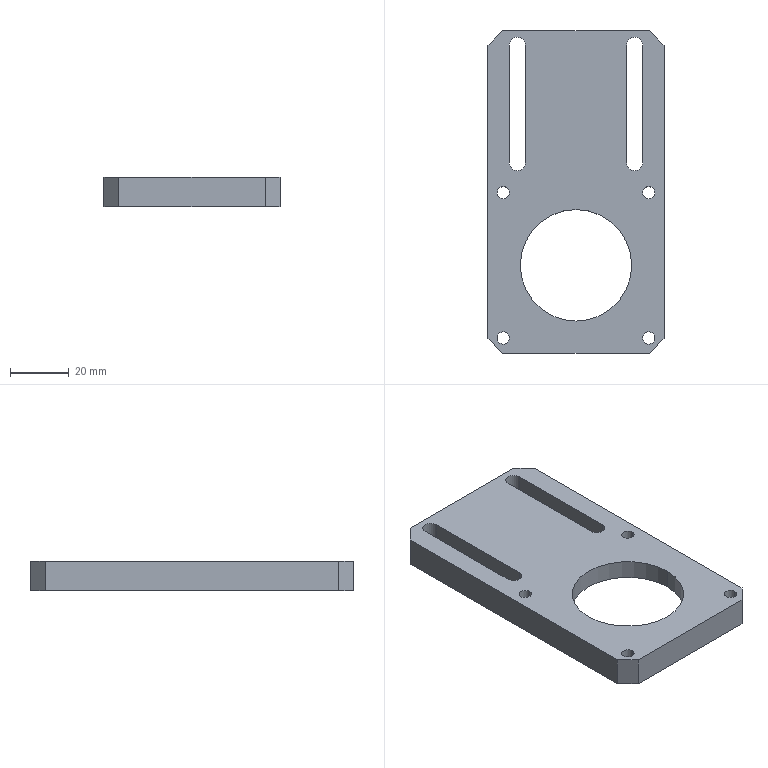Part | SolidWorks | features BaseBody 1 | 1 solid | 31 faces | box 60 x 110 x 10 mm | volume 45827 mm3 | cylinder 16 | plane 15 | commonest cylinder face diameters 4.2 x8 5.5 x4 38 x2 50 x2
STEP:
#1=CARTESIAN_POINT('',(26.849,-0.2513,10.));
#2=VERTEX_POINT('',#1);
#3=CARTESIAN_POINT('',(22.649,-0.2513,10.));
#4=VERTEX_POINT('',#3);
#5=CARTESIAN_POINT('',(24.749,-0.2513,10.));
#6=DIRECTION('',(0.,0.,-1.));
#7=DIRECTION('',(-1.,0.,0.));
#8=AXIS2_PLACEMENT_3D('',#5,#6,#7);
#9=CIRCLE('',#8,2.1);
#10=EDGE_CURVE('',#2,#4,#9,.T.);
#11=ORIENTED_EDGE('',*,*,#10,.F.);
#12=CARTESIAN_POINT('',(26.849,-0.2513,0.));
#13=VERTEX_POINT('',#12);
#14=CARTESIAN_POINT('',(26.849,-0.2513,0.));
#15=DIRECTION('',(0.,0.,-1.));
#16=VECTOR('',#15,1000.);
#17=LINE('',#14,#16);
#18=EDGE_CURVE('',#2,#13,#17,.T.);
#19=ORIENTED_EDGE('',*,*,#18,.T.);
#20=CARTESIAN_POINT('',(22.649,-0.2513,0.));
#21=VERTEX_POINT('',#20);
#22=CARTESIAN_POINT('',(24.749,-0.2513,0.));
#23=DIRECTION('',(0.,0.,-1.));
#24=DIRECTION('',(-1.,0.,0.));
#25=AXIS2_PLACEMENT_3D('',#22,#23,#24);
#26=CIRCLE('',#25,2.1);
#27=EDGE_CURVE('',#13,#21,#26,.T.);
#28=ORIENTED_EDGE('',*,*,#27,.T.);
#29=CARTESIAN_POINT('',(22.649,-0.2513,0.));
#30=DIRECTION('',(0.,0.,-1.));
#31=VECTOR('',#30,1000.);
#32=LINE('',#29,#31);
#33=EDGE_CURVE('',#4,#21,#32,.T.);
#34=ORIENTED_EDGE('',*,*,#33,.F.);
#35=EDGE_LOOP('',(#11,#19,#28,#34));
#36=FACE_OUTER_BOUND('',#35,.T.);
#37=CARTESIAN_POINT('',(24.749,-0.2513,0.));
#38=DIRECTION('',(0.,0.,-1.));
#39=DIRECTION('',(-1.,0.,0.));
#40=AXIS2_PLACEMENT_3D('',#37,#38,#39);
#41=CYLINDRICAL_SURFACE('',#40,2.1);
#42=ADVANCED_FACE('',(#36),#41,.F.);
#43=CARTESIAN_POINT('',(-22.649,-0.2513,10.));
#44=VERTEX_POINT('',#43);
#45=CARTESIAN_POINT('',(-26.849,-0.2513,10.));
#46=VERTEX_POINT('',#45);
#47=CARTESIAN_POINT('',(-24.749,-0.2513,10.));
#48=DIRECTION('',(0.,0.,-1.));
#49=DIRECTION('',(-1.,0.,0.));
#50=AXIS2_PLACEMENT_3D('',#47,#48,#49);
#51=CIRCLE('',#50,2.1);
#52=EDGE_CURVE('',#44,#46,#51,.T.);
#53=ORIENTED_EDGE('',*,*,#52,.F.);
#54=CARTESIAN_POINT('',(-22.649,-0.2513,0.));
#55=VERTEX_POINT('',#54);
#56=CARTESIAN_POINT('',(-22.649,-0.2513,0.));
#57=DIRECTION('',(0.,0.,-1.));
#58=VECTOR('',#57,1000.);
#59=LINE('',#56,#58);
#60=EDGE_CURVE('',#44,#55,#59,.T.);
#61=ORIENTED_EDGE('',*,*,#60,.T.);
#62=CARTESIAN_POINT('',(-26.849,-0.2513,0.));
#63=VERTEX_POINT('',#62);
#64=CARTESIAN_POINT('',(-24.749,-0.2513,0.));
#65=DIRECTION('',(0.,0.,-1.));
#66=DIRECTION('',(-1.,0.,0.));
#67=AXIS2_PLACEMENT_3D('',#64,#65,#66);
#68=CIRCLE('',#67,2.1);
#69=EDGE_CURVE('',#55,#63,#68,.T.);
#70=ORIENTED_EDGE('',*,*,#69,.T.);
#71=CARTESIAN_POINT('',(-26.849,-0.2513,0.));
#72=DIRECTION('',(0.,0.,-1.));
#73=VECTOR('',#72,1000.);
#74=LINE('',#71,#73);
#75=EDGE_CURVE('',#46,#63,#74,.T.);
#76=ORIENTED_EDGE('',*,*,#75,.F.);
#77=EDGE_LOOP('',(#53,#61,#70,#76));
#78=FACE_OUTER_BOUND('',#77,.T.);
#79=CARTESIAN_POINT('',(-24.749,-0.2513,0.));
#80=DIRECTION('',(0.,0.,-1.));
#81=DIRECTION('',(-1.,0.,0.));
#82=AXIS2_PLACEMENT_3D('',#79,#80,#81);
#83=CYLINDRICAL_SURFACE('',#82,2.1);
#84=ADVANCED_FACE('',(#78),#83,.F.);
#85=CARTESIAN_POINT('',(26.849,-49.749,10.));
#86=VERTEX_POINT('',#85);
#87=CARTESIAN_POINT('',(22.649,-49.749,10.));
#88=VERTEX_POINT('',#87);
#89=CARTESIAN_POINT('',(24.749,-49.749,10.));
#90=DIRECTION('',(0.,0.,-1.));
#91=DIRECTION('',(-1.,0.,0.));
#92=AXIS2_PLACEMENT_3D('',#89,#90,#91);
#93=CIRCLE('',#92,2.1);
#94=EDGE_CURVE('',#86,#88,#93,.T.);
#95=ORIENTED_EDGE('',*,*,#94,.F.);
#96=CARTESIAN_POINT('',(26.849,-49.749,0.));
#97=VERTEX_POINT('',#96);
#98=CARTESIAN_POINT('',(26.849,-49.749,0.));
#99=DIRECTION('',(0.,0.,-1.));
#100=VECTOR('',#99,1000.);
#101=LINE('',#98,#100);
#102=EDGE_CURVE('',#86,#97,#101,.T.);
#103=ORIENTED_EDGE('',*,*,#102,.T.);
#104=CARTESIAN_POINT('',(22.649,-49.749,0.));
#105=VERTEX_POINT('',#104);
#106=CARTESIAN_POINT('',(24.749,-49.749,0.));
#107=DIRECTION('',(0.,0.,-1.));
#108=DIRECTION('',(-1.,0.,0.));
#109=AXIS2_PLACEMENT_3D('',#106,#107,#108);
#110=CIRCLE('',#109,2.1);
#111=EDGE_CURVE('',#97,#105,#110,.T.);
#112=ORIENTED_EDGE('',*,*,#111,.T.);
#113=CARTESIAN_POINT('',(22.649,-49.749,0.));
#114=DIRECTION('',(0.,0.,-1.));
#115=VECTOR('',#114,1000.);
#116=LINE('',#113,#115);
#117=EDGE_CURVE('',#88,#105,#116,.T.);
#118=ORIENTED_EDGE('',*,*,#117,.F.);
#119=EDGE_LOOP('',(#95,#103,#112,#118));
#120=FACE_OUTER_BOUND('',#119,.T.);
#121=CARTESIAN_POINT('',(24.749,-49.749,0.));
#122=DIRECTION('',(0.,0.,-1.));
#123=DIRECTION('',(-1.,0.,0.));
#124=AXIS2_PLACEMENT_3D('',#121,#122,#123);
#125=CYLINDRICAL_SURFACE('',#124,2.1);
#126=ADVANCED_FACE('',(#120),#125,.F.);
#127=CARTESIAN_POINT('',(-22.649,-49.749,10.));
#128=VERTEX_POINT('',#127);
#129=CARTESIAN_POINT('',(-26.849,-49.749,10.));
#130=VERTEX_POINT('',#129);
#131=CARTESIAN_POINT('',(-24.749,-49.749,10.));
#132=DIRECTION('',(0.,0.,-1.));
#133=DIRECTION('',(-1.,0.,0.));
#134=AXIS2_PLACEMENT_3D('',#131,#132,#133);
#135=CIRCLE('',#134,2.1);
#136=EDGE_CURVE('',#128,#130,#135,.T.);
#137=ORIENTED_EDGE('',*,*,#136,.F.);
#138=CARTESIAN_POINT('',(-22.649,-49.749,0.));
#139=VERTEX_POINT('',#138);
#140=CARTESIAN_POINT('',(-22.649,-49.749,0.));
#141=DIRECTION('',(0.,0.,-1.));
#142=VECTOR('',#141,1000.);
#143=LINE('',#140,#142);
#144=EDGE_CURVE('',#128,#139,#143,.T.);
#145=ORIENTED_EDGE('',*,*,#144,.T.);
#146=CARTESIAN_POINT('',(-26.849,-49.749,0.));
#147=VERTEX_POINT('',#146);
#148=CARTESIAN_POINT('',(-24.749,-49.749,0.));
#149=DIRECTION('',(0.,0.,-1.));
#150=DIRECTION('',(-1.,0.,0.));
#151=AXIS2_PLACEMENT_3D('',#148,#149,#150);
#152=CIRCLE('',#151,2.1);
#153=EDGE_CURVE('',#139,#147,#152,.T.);
#154=ORIENTED_EDGE('',*,*,#153,.T.);
#155=CARTESIAN_POINT('',(-26.849,-49.749,0.));
#156=DIRECTION('',(0.,0.,-1.));
#157=VECTOR('',#156,1000.);
#158=LINE('',#155,#157);
#159=EDGE_CURVE('',#130,#147,#158,.T.);
#160=ORIENTED_EDGE('',*,*,#159,.F.);
#161=EDGE_LOOP('',(#137,#145,#154,#160));
#162=FACE_OUTER_BOUND('',#161,.T.);
#163=CARTESIAN_POINT('',(-24.749,-49.749,0.));
#164=DIRECTION('',(0.,0.,-1.));
#165=DIRECTION('',(-1.,0.,0.));
#166=AXIS2_PLACEMENT_3D('',#163,#164,#165);
#167=CYLINDRICAL_SURFACE('',#166,2.1);
#168=ADVANCED_FACE('',(#162),#167,.F.);
#169=CARTESIAN_POINT('',(19.,-25.,10.));
#170=VERTEX_POINT('',#169);
#171=CARTESIAN_POINT('',(-19.,-25.,10.));
#172=VERTEX_POINT('',#171);
#173=CARTESIAN_POINT('',(0.,-25.,10.));
#174=DIRECTION('',(0.,0.,-1.));
#175=DIRECTION('',(-1.,0.,0.));
#176=AXIS2_PLACEMENT_3D('',#173,#174,#175);
#177=CIRCLE('',#176,19.);
#178=EDGE_CURVE('',#170,#172,#177,.T.);
#179=ORIENTED_EDGE('',*,*,#178,.F.);
#180=CARTESIAN_POINT('',(19.,-25.,3.5));
#181=VERTEX_POINT('',#180);
#182=CARTESIAN_POINT('',(19.,-25.,10.));
#183=DIRECTION('',(0.,0.,-1.));
#184=VECTOR('',#183,1000.);
#185=LINE('',#182,#184);
#186=EDGE_CURVE('',#170,#181,#185,.T.);
#187=ORIENTED_EDGE('',*,*,#186,.T.);
#188=CARTESIAN_POINT('',(-19.,-25.,3.5));
#189=VERTEX_POINT('',#188);
#190=CARTESIAN_POINT('',(0.,-25.,3.5));
#191=DIRECTION('',(0.,0.,-1.));
#192=DIRECTION('',(-1.,0.,0.));
#193=AXIS2_PLACEMENT_3D('',#190,#191,#192);
#194=CIRCLE('',#193,19.);
#195=EDGE_CURVE('',#181,#189,#194,.T.);
#196=ORIENTED_EDGE('',*,*,#195,.T.);
#197=CARTESIAN_POINT('',(-19.,-25.,10.));
#198=DIRECTION('',(0.,0.,-1.));
#199=VECTOR('',#198,1000.);
#200=LINE('',#197,#199);
#201=EDGE_CURVE('',#172,#189,#200,.T.);
#202=ORIENTED_EDGE('',*,*,#201,.F.);
#203=EDGE_LOOP('',(#179,#187,#196,#202));
#204=FACE_OUTER_BOUND('',#203,.T.);
#205=CARTESIAN_POINT('',(0.,-25.,10.));
#206=DIRECTION('',(0.,0.,-1.));
#207=DIRECTION('',(-1.,0.,0.));
#208=AXIS2_PLACEMENT_3D('',#205,#206,#207);
#209=CYLINDRICAL_SURFACE('',#208,19.);
#210=ADVANCED_FACE('',(#204),#209,.F.);
#211=CARTESIAN_POINT('',(25.,-25.,3.5));
#212=VERTEX_POINT('',#211);
#213=CARTESIAN_POINT('',(-25.,-25.,3.5));
#214=VERTEX_POINT('',#213);
#215=CARTESIAN_POINT('',(0.,-25.,3.5));
#216=DIRECTION('',(0.,0.,-1.));
#217=DIRECTION('',(-1.,0.,0.));
#218=AXIS2_PLACEMENT_3D('',#215,#216,#217);
#219=CIRCLE('',#218,25.);
#220=EDGE_CURVE('',#212,#214,#219,.T.);
#221=ORIENTED_EDGE('',*,*,#220,.F.);
#222=CARTESIAN_POINT('',(25.,-25.,0.));
#223=VERTEX_POINT('',#222);
#224=CARTESIAN_POINT('',(25.,-25.,3.5));
#225=DIRECTION('',(0.,0.,-1.));
#226=VECTOR('',#225,1000.);
#227=LINE('',#224,#226);
#228=EDGE_CURVE('',#212,#223,#227,.T.);
#229=ORIENTED_EDGE('',*,*,#228,.T.);
#230=CARTESIAN_POINT('',(-25.,-25.,0.));
#231=VERTEX_POINT('',#230);
#232=CARTESIAN_POINT('',(0.,-25.,0.));
#233=DIRECTION('',(0.,0.,-1.));
#234=DIRECTION('',(-1.,0.,0.));
#235=AXIS2_PLACEMENT_3D('',#232,#233,#234);
#236=CIRCLE('',#235,25.);
#237=EDGE_CURVE('',#223,#231,#236,.T.);
#238=ORIENTED_EDGE('',*,*,#237,.T.);
#239=CARTESIAN_POINT('',(-25.,-25.,3.5));
#240=DIRECTION('',(0.,0.,-1.));
#241=VECTOR('',#240,1000.);
#242=LINE('',#239,#241);
#243=EDGE_CURVE('',#214,#231,#242,.T.);
#244=ORIENTED_EDGE('',*,*,#243,.F.);
#245=EDGE_LOOP('',(#221,#229,#238,#244));
#246=FACE_OUTER_BOUND('',#245,.T.);
#247=CARTESIAN_POINT('',(0.,-25.,3.5));
#248=DIRECTION('',(0.,0.,-1.));
#249=DIRECTION('',(-1.,0.,0.));
#250=AXIS2_PLACEMENT_3D('',#247,#248,#249);
#251=CYLINDRICAL_SURFACE('',#250,25.);
#252=ADVANCED_FACE('',(#246),#251,.F.);
#253=CARTESIAN_POINT('',(-30.,50.,10.));
#254=VERTEX_POINT('',#253);
#255=CARTESIAN_POINT('',(-30.,-50.,10.));
#256=VERTEX_POINT('',#255);
#257=CARTESIAN_POINT('',(-30.,55.,10.));
#258=DIRECTION('',(0.,-1.,0.));
#259=VECTOR('',#258,1000.);
#260=LINE('',#257,#259);
#261=EDGE_CURVE('',#254,#256,#260,.T.);
#262=ORIENTED_EDGE('',*,*,#261,.F.);
#263=CARTESIAN_POINT('',(-30.,50.,0.));
#264=VERTEX_POINT('',#263);
#265=CARTESIAN_POINT('',(-30.,50.,10.));
#266=DIRECTION('',(0.,0.,-1.));
#267=VECTOR('',#266,1000.);
#268=LINE('',#265,#267);
#269=EDGE_CURVE('',#254,#264,#268,.T.);
#270=ORIENTED_EDGE('',*,*,#269,.T.);
#271=CARTESIAN_POINT('',(-30.,-50.,0.));
#272=VERTEX_POINT('',#271);
#273=CARTESIAN_POINT('',(-30.,55.,0.));
#274=DIRECTION('',(0.,-1.,0.));
#275=VECTOR('',#274,1000.);
#276=LINE('',#273,#275);
#277=EDGE_CURVE('',#264,#272,#276,.T.);
#278=ORIENTED_EDGE('',*,*,#277,.T.);
#279=CARTESIAN_POINT('',(-30.,-50.,10.));
#280=DIRECTION('',(0.,0.,1.));
#281=VECTOR('',#280,1000.);
#282=LINE('',#279,#281);
#283=EDGE_CURVE('',#272,#256,#282,.T.);
#284=ORIENTED_EDGE('',*,*,#283,.T.);
#285=EDGE_LOOP('',(#262,#270,#278,#284));
#286=FACE_OUTER_BOUND('',#285,.T.);
#287=CARTESIAN_POINT('',(-30.,55.,10.));
#288=DIRECTION('',(1.,0.,0.));
#289=DIRECTION('',(0.,1.,0.));
#290=AXIS2_PLACEMENT_3D('',#287,#288,#289);
#291=PLANE('',#290);
#292=ADVANCED_FACE('',(#286),#291,.F.);
#293=CARTESIAN_POINT('',(-25.,-55.,0.));
#294=VERTEX_POINT('',#293);
#295=CARTESIAN_POINT('',(25.,-55.,0.));
#296=VERTEX_POINT('',#295);
#297=CARTESIAN_POINT('',(30.,-55.,0.));
#298=DIRECTION('',(1.,0.,0.));
#299=VECTOR('',#298,1000.);
#300=LINE('',#297,#299);
#301=EDGE_CURVE('',#294,#296,#300,.T.);
#302=ORIENTED_EDGE('',*,*,#301,.T.);
#303=CARTESIAN_POINT('',(25.,-55.,10.));
#304=VERTEX_POINT('',#303);
#305=CARTESIAN_POINT('',(25.,-55.,10.));
#306=DIRECTION('',(0.,0.,1.));
#307=VECTOR('',#306,1000.);
#308=LINE('',#305,#307);
#309=EDGE_CURVE('',#296,#304,#308,.T.);
#310=ORIENTED_EDGE('',*,*,#309,.T.);
#311=CARTESIAN_POINT('',(-25.,-55.,10.));
#312=VERTEX_POINT('',#311);
#313=CARTESIAN_POINT('',(30.,-55.,10.));
#314=DIRECTION('',(1.,0.,0.));
#315=VECTOR('',#314,1000.);
#316=LINE('',#313,#315);
#317=EDGE_CURVE('',#312,#304,#316,.T.);
#318=ORIENTED_EDGE('',*,*,#317,.F.);
#319=CARTESIAN_POINT('',(-25.,-55.,10.));
#320=DIRECTION('',(0.,0.,-1.));
#321=VECTOR('',#320,1000.);
#322=LINE('',#319,#321);
#323=EDGE_CURVE('',#312,#294,#322,.T.);
#324=ORIENTED_EDGE('',*,*,#323,.T.);
#325=EDGE_LOOP('',(#302,#310,#318,#324));
#326=FACE_OUTER_BOUND('',#325,.T.);
#327=CARTESIAN_POINT('',(30.,-55.,10.));
#328=DIRECTION('',(0.,1.,0.));
#329=DIRECTION('',(-1.,0.,0.));
#330=AXIS2_PLACEMENT_3D('',#327,#328,#329);
#331=PLANE('',#330);
#332=ADVANCED_FACE('',(#326),#331,.F.);
#333=CARTESIAN_POINT('',(30.,-50.,0.));
#334=VERTEX_POINT('',#333);
#335=CARTESIAN_POINT('',(30.,50.,0.));
#336=VERTEX_POINT('',#335);
#337=CARTESIAN_POINT('',(30.,55.,0.));
#338=DIRECTION('',(0.,1.,0.));
#339=VECTOR('',#338,1000.);
#340=LINE('',#337,#339);
#341=EDGE_CURVE('',#334,#336,#340,.T.);
#342=ORIENTED_EDGE('',*,*,#341,.T.);
#343=CARTESIAN_POINT('',(30.,50.,10.));
#344=VERTEX_POINT('',#343);
#345=CARTESIAN_POINT('',(30.,50.,10.));
#346=DIRECTION('',(0.,0.,1.));
#347=VECTOR('',#346,1000.);
#348=LINE('',#345,#347);
#349=EDGE_CURVE('',#336,#344,#348,.T.);
#350=ORIENTED_EDGE('',*,*,#349,.T.);
#351=CARTESIAN_POINT('',(30.,-50.,10.));
#352=VERTEX_POINT('',#351);
#353=CARTESIAN_POINT('',(30.,55.,10.));
#354=DIRECTION('',(0.,1.,0.));
#355=VECTOR('',#354,1000.);
#356=LINE('',#353,#355);
#357=EDGE_CURVE('',#352,#344,#356,.T.);
#358=ORIENTED_EDGE('',*,*,#357,.F.);
#359=CARTESIAN_POINT('',(30.,-50.,10.));
#360=DIRECTION('',(0.,0.,-1.));
#361=VECTOR('',#360,1000.);
#362=LINE('',#359,#361);
#363=EDGE_CURVE('',#352,#334,#362,.T.);
#364=ORIENTED_EDGE('',*,*,#363,.T.);
#365=EDGE_LOOP('',(#342,#350,#358,#364));
#366=FACE_OUTER_BOUND('',#365,.T.);
#367=CARTESIAN_POINT('',(30.,55.,10.));
#368=DIRECTION('',(-1.,0.,0.));
#369=DIRECTION('',(0.,-1.,0.));
#370=AXIS2_PLACEMENT_3D('',#367,#368,#369);
#371=PLANE('',#370);
#372=ADVANCED_FACE('',(#366),#371,.F.);
#373=CARTESIAN_POINT('',(25.,55.,10.));
#374=VERTEX_POINT('',#373);
#375=CARTESIAN_POINT('',(-25.,55.,10.));
#376=VERTEX_POINT('',#375);
#377=CARTESIAN_POINT('',(30.,55.,10.));
#378=DIRECTION('',(-1.,0.,0.));
#379=VECTOR('',#378,1000.);
#380=LINE('',#377,#379);
#381=EDGE_CURVE('',#374,#376,#380,.T.);
#382=ORIENTED_EDGE('',*,*,#381,.F.);
#383=CARTESIAN_POINT('',(25.,55.,0.));
#384=VERTEX_POINT('',#383);
#385=CARTESIAN_POINT('',(25.,55.,10.));
#386=DIRECTION('',(0.,0.,-1.));
#387=VECTOR('',#386,1000.);
#388=LINE('',#385,#387);
#389=EDGE_CURVE('',#374,#384,#388,.T.);
#390=ORIENTED_EDGE('',*,*,#389,.T.);
#391=CARTESIAN_POINT('',(-25.,55.,0.));
#392=VERTEX_POINT('',#391);
#393=CARTESIAN_POINT('',(30.,55.,0.));
#394=DIRECTION('',(-1.,0.,0.));
#395=VECTOR('',#394,1000.);
#396=LINE('',#393,#395);
#397=EDGE_CURVE('',#384,#392,#396,.T.);
#398=ORIENTED_EDGE('',*,*,#397,.T.);
#399=CARTESIAN_POINT('',(-25.,55.,10.));
#400=DIRECTION('',(0.,0.,1.));
#401=VECTOR('',#400,1000.);
#402=LINE('',#399,#401);
#403=EDGE_CURVE('',#392,#376,#402,.T.);
#404=ORIENTED_EDGE('',*,*,#403,.T.);
#405=EDGE_LOOP('',(#382,#390,#398,#404));
#406=FACE_OUTER_BOUND('',#405,.T.);
#407=CARTESIAN_POINT('',(30.,55.,10.));
#408=DIRECTION('',(0.,-1.,0.));
#409=DIRECTION('',(1.,0.,0.));
#410=AXIS2_PLACEMENT_3D('',#407,#408,#409);
#411=PLANE('',#410);
#412=ADVANCED_FACE('',(#406),#411,.F.);
#413=CARTESIAN_POINT('',(24.749,-0.2513,10.));
#414=DIRECTION('',(0.,0.,-1.));
#415=DIRECTION('',(-1.,0.,0.));
#416=AXIS2_PLACEMENT_3D('',#413,#414,#415);
#417=CIRCLE('',#416,2.1);
#418=EDGE_CURVE('',#4,#2,#417,.T.);
#419=ORIENTED_EDGE('',*,*,#418,.T.);
#420=ORIENTED_EDGE('',*,*,#10,.T.);
#421=EDGE_LOOP('',(#419,#420));
#422=FACE_BOUND('',#421,.T.);
#423=CARTESIAN_POINT('',(-24.749,-0.2513,10.));
#424=DIRECTION('',(0.,0.,-1.));
#425=DIRECTION('',(-1.,0.,0.));
#426=AXIS2_PLACEMENT_3D('',#423,#424,#425);
#427=CIRCLE('',#426,2.1);
#428=EDGE_CURVE('',#46,#44,#427,.T.);
#429=ORIENTED_EDGE('',*,*,#428,.T.);
#430=ORIENTED_EDGE('',*,*,#52,.T.);
#431=EDGE_LOOP('',(#429,#430));
#432=FACE_BOUND('',#431,.T.);
#433=CARTESIAN_POINT('',(24.749,-49.749,10.));
#434=DIRECTION('',(0.,0.,-1.));
#435=DIRECTION('',(-1.,0.,0.));
#436=AXIS2_PLACEMENT_3D('',#433,#434,#435);
#437=CIRCLE('',#436,2.1);
#438=EDGE_CURVE('',#88,#86,#437,.T.);
#439=ORIENTED_EDGE('',*,*,#438,.T.);
#440=ORIENTED_EDGE('',*,*,#94,.T.);
#441=EDGE_LOOP('',(#439,#440));
#442=FACE_BOUND('',#441,.T.);
#443=CARTESIAN_POINT('',(-24.749,-49.749,10.));
#444=DIRECTION('',(0.,0.,-1.));
#445=DIRECTION('',(-1.,0.,0.));
#446=AXIS2_PLACEMENT_3D('',#443,#444,#445);
#447=CIRCLE('',#446,2.1);
#448=EDGE_CURVE('',#130,#128,#447,.T.);
#449=ORIENTED_EDGE('',*,*,#448,.T.);
#450=ORIENTED_EDGE('',*,*,#136,.T.);
#451=EDGE_LOOP('',(#449,#450));
#452=FACE_BOUND('',#451,.T.);
#453=CARTESIAN_POINT('',(17.25,50.,10.));
#454=VERTEX_POINT('',#453);
#455=CARTESIAN_POINT('',(17.25,10.,10.));
#456=VERTEX_POINT('',#455);
#457=CARTESIAN_POINT('',(17.25,50.,10.));
#458=DIRECTION('',(0.,-1.,0.));
#459=VECTOR('',#458,1000.);
#460=LINE('',#457,#459);
#461=EDGE_CURVE('',#454,#456,#460,.T.);
#462=ORIENTED_EDGE('',*,*,#461,.F.);
#463=CARTESIAN_POINT('',(22.75,50.,10.));
#464=VERTEX_POINT('',#463);
#465=CARTESIAN_POINT('',(20.,50.,10.));
#466=DIRECTION('',(0.,0.,1.));
#467=DIRECTION('',(-1.,0.,0.));
#468=AXIS2_PLACEMENT_3D('',#465,#466,#467);
#469=CIRCLE('',#468,2.75);
#470=EDGE_CURVE('',#464,#454,#469,.T.);
#471=ORIENTED_EDGE('',*,*,#470,.F.);
#472=CARTESIAN_POINT('',(22.75,10.,10.));
#473=VERTEX_POINT('',#472);
#474=CARTESIAN_POINT('',(22.75,50.,10.));
#475=DIRECTION('',(0.,1.,0.));
#476=VECTOR('',#475,1000.);
#477=LINE('',#474,#476);
#478=EDGE_CURVE('',#473,#464,#477,.T.);
#479=ORIENTED_EDGE('',*,*,#478,.F.);
#480=CARTESIAN_POINT('',(20.,10.,10.));
#481=DIRECTION('',(0.,0.,1.));
#482=DIRECTION('',(-1.,0.,0.));
#483=AXIS2_PLACEMENT_3D('',#480,#481,#482);
#484=CIRCLE('',#483,2.75);
#485=EDGE_CURVE('',#456,#473,#484,.T.);
#486=ORIENTED_EDGE('',*,*,#485,.F.);
#487=EDGE_LOOP('',(#462,#471,#479,#486));
#488=FACE_BOUND('',#487,.T.);
#489=CARTESIAN_POINT('',(-22.75,50.,10.));
#490=VERTEX_POINT('',#489);
#491=CARTESIAN_POINT('',(-22.75,10.,10.));
#492=VERTEX_POINT('',#491);
#493=CARTESIAN_POINT('',(-22.75,50.,10.));
#494=DIRECTION('',(0.,-1.,0.));
#495=VECTOR('',#494,1000.);
#496=LINE('',#493,#495);
#497=EDGE_CURVE('',#490,#492,#496,.T.);
#498=ORIENTED_EDGE('',*,*,#497,.F.);
#499=CARTESIAN_POINT('',(-17.25,50.,10.));
#500=VERTEX_POINT('',#499);
#501=CARTESIAN_POINT('',(-20.,50.,10.));
#502=DIRECTION('',(0.,0.,1.));
#503=DIRECTION('',(1.,0.,0.));
#504=AXIS2_PLACEMENT_3D('',#501,#502,#503);
#505=CIRCLE('',#504,2.75);
#506=EDGE_CURVE('',#500,#490,#505,.T.);
#507=ORIENTED_EDGE('',*,*,#506,.F.);
#508=CARTESIAN_POINT('',(-17.25,10.,10.));
#509=VERTEX_POINT('',#508);
#510=CARTESIAN_POINT('',(-17.25,50.,10.));
#511=DIRECTION('',(0.,1.,0.));
#512=VECTOR('',#511,1000.);
#513=LINE('',#510,#512);
#514=EDGE_CURVE('',#509,#500,#513,.T.);
#515=ORIENTED_EDGE('',*,*,#514,.F.);
#516=CARTESIAN_POINT('',(-20.,10.,10.));
#517=DIRECTION('',(0.,0.,1.));
#518=DIRECTION('',(1.,0.,0.));
#519=AXIS2_PLACEMENT_3D('',#516,#517,#518);
#520=CIRCLE('',#519,2.75);
#521=EDGE_CURVE('',#492,#509,#520,.T.);
#522=ORIENTED_EDGE('',*,*,#521,.F.);
#523=EDGE_LOOP('',(#498,#507,#515,#522));
#524=FACE_BOUND('',#523,.T.);
#525=CARTESIAN_POINT('',(0.,-25.,10.));
#526=DIRECTION('',(0.,0.,-1.));
#527=DIRECTION('',(-1.,0.,0.));
#528=AXIS2_PLACEMENT_3D('',#525,#526,#527);
#529=CIRCLE('',#528,19.);
#530=EDGE_CURVE('',#172,#170,#529,.T.);
#531=ORIENTED_EDGE('',*,*,#530,.T.);
#532=ORIENTED_EDGE('',*,*,#178,.T.);
#533=EDGE_LOOP('',(#531,#532));
#534=FACE_BOUND('',#533,.T.);
#535=ORIENTED_EDGE('',*,*,#357,.T.);
#536=CARTESIAN_POINT('',(25.,55.,10.));
#537=DIRECTION('',(-0.7071,0.7071,0.));
#538=VECTOR('',#537,1000.);
#539=LINE('',#536,#538);
#540=EDGE_CURVE('',#344,#374,#539,.T.);
#541=ORIENTED_EDGE('',*,*,#540,.T.);
#542=ORIENTED_EDGE('',*,*,#381,.T.);
#543=CARTESIAN_POINT('',(-30.,50.,10.));
#544=DIRECTION('',(-0.7071,-0.7071,0.));
#545=VECTOR('',#544,1000.);
#546=LINE('',#543,#545);
#547=EDGE_CURVE('',#376,#254,#546,.T.);
#548=ORIENTED_EDGE('',*,*,#547,.T.);
#549=ORIENTED_EDGE('',*,*,#261,.T.);
#550=CARTESIAN_POINT('',(-25.,-55.,10.));
#551=DIRECTION('',(0.7071,-0.7071,0.));
#552=VECTOR('',#551,1000.);
#553=LINE('',#550,#552);
#554=EDGE_CURVE('',#256,#312,#553,.T.);
#555=ORIENTED_EDGE('',*,*,#554,.T.);
#556=ORIENTED_EDGE('',*,*,#317,.T.);
#557=CARTESIAN_POINT('',(30.,-50.,10.));
#558=DIRECTION('',(0.7071,0.7071,0.));
#559=VECTOR('',#558,1000.);
#560=LINE('',#557,#559);
#561=EDGE_CURVE('',#304,#352,#560,.T.);
#562=ORIENTED_EDGE('',*,*,#561,.T.);
#563=EDGE_LOOP('',(#535,#541,#542,#548,#549,#555,#556,#562));
#564=FACE_OUTER_BOUND('',#563,.T.);
#565=CARTESIAN_POINT('',(0.,0.,10.));
#566=DIRECTION('',(0.,0.,-1.));
#567=DIRECTION('',(-1.,0.,0.));
#568=AXIS2_PLACEMENT_3D('',#565,#566,#567);
#569=PLANE('',#568);
#570=ADVANCED_FACE('',(#422,#432,#442,#452,#488,#524,#534,#564),#569,.F.);
#571=CARTESIAN_POINT('',(24.749,-0.2513,0.));
#572=DIRECTION('',(0.,0.,-1.));
#573=DIRECTION('',(-1.,0.,0.));
#574=AXIS2_PLACEMENT_3D('',#571,#572,#573);
#575=CIRCLE('',#574,2.1);
#576=EDGE_CURVE('',#21,#13,#575,.T.);
#577=ORIENTED_EDGE('',*,*,#576,.F.);
#578=ORIENTED_EDGE('',*,*,#27,.F.);
#579=EDGE_LOOP('',(#577,#578));
#580=FACE_BOUND('',#579,.T.);
#581=CARTESIAN_POINT('',(-24.749,-0.2513,0.));
#582=DIRECTION('',(0.,0.,-1.));
#583=DIRECTION('',(-1.,0.,0.));
#584=AXIS2_PLACEMENT_3D('',#581,#582,#583);
#585=CIRCLE('',#584,2.1);
#586=EDGE_CURVE('',#63,#55,#585,.T.);
#587=ORIENTED_EDGE('',*,*,#586,.F.);
#588=ORIENTED_EDGE('',*,*,#69,.F.);
#589=EDGE_LOOP('',(#587,#588));
#590=FACE_BOUND('',#589,.T.);
#591=CARTESIAN_POINT('',(24.749,-49.749,0.));
#592=DIRECTION('',(0.,0.,-1.));
#593=DIRECTION('',(-1.,0.,0.));
#594=AXIS2_PLACEMENT_3D('',#591,#592,#593);
#595=CIRCLE('',#594,2.1);
#596=EDGE_CURVE('',#105,#97,#595,.T.);
#597=ORIENTED_EDGE('',*,*,#596,.F.);
#598=ORIENTED_EDGE('',*,*,#111,.F.);
#599=EDGE_LOOP('',(#597,#598));
#600=FACE_BOUND('',#599,.T.);
#601=CARTESIAN_POINT('',(-24.749,-49.749,0.));
#602=DIRECTION('',(0.,0.,-1.));
#603=DIRECTION('',(-1.,0.,0.));
#604=AXIS2_PLACEMENT_3D('',#601,#602,#603);
#605=CIRCLE('',#604,2.1);
#606=EDGE_CURVE('',#147,#139,#605,.T.);
#607=ORIENTED_EDGE('',*,*,#606,.F.);
#608=ORIENTED_EDGE('',*,*,#153,.F.);
#609=EDGE_LOOP('',(#607,#608));
#610=FACE_BOUND('',#609,.T.);
#611=CARTESIAN_POINT('',(22.75,50.,0.));
#612=VERTEX_POINT('',#611);
#613=CARTESIAN_POINT('',(17.25,50.,0.));
#614=VERTEX_POINT('',#613);
#615=CARTESIAN_POINT('',(20.,50.,0.));
#616=DIRECTION('',(0.,0.,1.));
#617=DIRECTION('',(-1.,0.,0.));
#618=AXIS2_PLACEMENT_3D('',#615,#616,#617);
#619=CIRCLE('',#618,2.75);
#620=EDGE_CURVE('',#612,#614,#619,.T.);
#621=ORIENTED_EDGE('',*,*,#620,.T.);
#622=CARTESIAN_POINT('',(17.25,10.,0.));
#623=VERTEX_POINT('',#622);
#624=CARTESIAN_POINT('',(17.25,50.,0.));
#625=DIRECTION('',(0.,-1.,0.));
#626=VECTOR('',#625,1000.);
#627=LINE('',#624,#626);
#628=EDGE_CURVE('',#614,#623,#627,.T.);
#629=ORIENTED_EDGE('',*,*,#628,.T.);
#630=CARTESIAN_POINT('',(22.75,10.,0.));
#631=VERTEX_POINT('',#630);
#632=CARTESIAN_POINT('',(20.,10.,0.));
#633=DIRECTION('',(0.,0.,1.));
#634=DIRECTION('',(-1.,0.,0.));
#635=AXIS2_PLACEMENT_3D('',#632,#633,#634);
#636=CIRCLE('',#635,2.75);
#637=EDGE_CURVE('',#623,#631,#636,.T.);
#638=ORIENTED_EDGE('',*,*,#637,.T.);
#639=CARTESIAN_POINT('',(22.75,50.,0.));
#640=DIRECTION('',(0.,1.,0.));
#641=VECTOR('',#640,1000.);
#642=LINE('',#639,#641);
#643=EDGE_CURVE('',#631,#612,#642,.T.);
#644=ORIENTED_EDGE('',*,*,#643,.T.);
#645=EDGE_LOOP('',(#621,#629,#638,#644));
#646=FACE_BOUND('',#645,.T.);
#647=CARTESIAN_POINT('',(-17.25,50.,0.));
#648=VERTEX_POINT('',#647);
#649=CARTESIAN_POINT('',(-22.75,50.,0.));
#650=VERTEX_POINT('',#649);
#651=CARTESIAN_POINT('',(-20.,50.,0.));
#652=DIRECTION('',(0.,0.,1.));
#653=DIRECTION('',(1.,0.,0.));
#654=AXIS2_PLACEMENT_3D('',#651,#652,#653);
#655=CIRCLE('',#654,2.75);
#656=EDGE_CURVE('',#648,#650,#655,.T.);
#657=ORIENTED_EDGE('',*,*,#656,.T.);
#658=CARTESIAN_POINT('',(-22.75,10.,0.));
#659=VERTEX_POINT('',#658);
#660=CARTESIAN_POINT('',(-22.75,50.,0.));
#661=DIRECTION('',(0.,-1.,0.));
#662=VECTOR('',#661,1000.);
#663=LINE('',#660,#662);
#664=EDGE_CURVE('',#650,#659,#663,.T.);
#665=ORIENTED_EDGE('',*,*,#664,.T.);
#666=CARTESIAN_POINT('',(-17.25,10.,0.));
#667=VERTEX_POINT('',#666);
#668=CARTESIAN_POINT('',(-20.,10.,0.));
#669=DIRECTION('',(0.,0.,1.));
#670=DIRECTION('',(1.,0.,0.));
#671=AXIS2_PLACEMENT_3D('',#668,#669,#670);
#672=CIRCLE('',#671,2.75);
#673=EDGE_CURVE('',#659,#667,#672,.T.);
#674=ORIENTED_EDGE('',*,*,#673,.T.);
#675=CARTESIAN_POINT('',(-17.25,50.,0.));
#676=DIRECTION('',(0.,1.,0.));
#677=VECTOR('',#676,1000.);
#678=LINE('',#675,#677);
#679=EDGE_CURVE('',#667,#648,#678,.T.);
#680=ORIENTED_EDGE('',*,*,#679,.T.);
#681=EDGE_LOOP('',(#657,#665,#674,#680));
#682=FACE_BOUND('',#681,.T.);
#683=CARTESIAN_POINT('',(0.,-25.,0.));
#684=DIRECTION('',(0.,0.,-1.));
#685=DIRECTION('',(-1.,0.,0.));
#686=AXIS2_PLACEMENT_3D('',#683,#684,#685);
#687=CIRCLE('',#686,25.);
#688=EDGE_CURVE('',#231,#223,#687,.T.);
#689=ORIENTED_EDGE('',*,*,#688,.F.);
#690=ORIENTED_EDGE('',*,*,#237,.F.);
#691=EDGE_LOOP('',(#689,#690));
#692=FACE_BOUND('',#691,.T.);
#693=ORIENTED_EDGE('',*,*,#397,.F.);
#694=CARTESIAN_POINT('',(40.,40.,0.));
#695=DIRECTION('',(0.7071,-0.7071,0.));
#696=VECTOR('',#695,1000.);
#697=LINE('',#694,#696);
#698=EDGE_CURVE('',#384,#336,#697,.T.);
#699=ORIENTED_EDGE('',*,*,#698,.T.);
#700=ORIENTED_EDGE('',*,*,#341,.F.);
#701=CARTESIAN_POINT('',(40.,-40.,0.));
#702=DIRECTION('',(-0.7071,-0.7071,0.));
#703=VECTOR('',#702,1000.);
#704=LINE('',#701,#703);
#705=EDGE_CURVE('',#334,#296,#704,.T.);
#706=ORIENTED_EDGE('',*,*,#705,.T.);
#707=ORIENTED_EDGE('',*,*,#301,.F.);
#708=CARTESIAN_POINT('',(-40.,-40.,0.));
#709=DIRECTION('',(-0.7071,0.7071,0.));
#710=VECTOR('',#709,1000.);
#711=LINE('',#708,#710);
#712=EDGE_CURVE('',#294,#272,#711,.T.);
#713=ORIENTED_EDGE('',*,*,#712,.T.);
#714=ORIENTED_EDGE('',*,*,#277,.F.);
#715=CARTESIAN_POINT('',(-40.,40.,0.));
#716=DIRECTION('',(0.7071,0.7071,0.));
#717=VECTOR('',#716,1000.);
#718=LINE('',#715,#717);
#719=EDGE_CURVE('',#264,#392,#718,.T.);
#720=ORIENTED_EDGE('',*,*,#719,.T.);
#721=EDGE_LOOP('',(#693,#699,#700,#706,#707,#713,#714,#720));
#722=FACE_OUTER_BOUND('',#721,.T.);
#723=CARTESIAN_POINT('',(0.,0.,0.));
#724=DIRECTION('',(0.,0.,-1.));
#725=DIRECTION('',(-1.,0.,0.));
#726=AXIS2_PLACEMENT_3D('',#723,#724,#725);
#727=PLANE('',#726);
#728=ADVANCED_FACE('',(#580,#590,#600,#610,#646,#682,#692,#722),#727,.T.);
#729=ORIENTED_EDGE('',*,*,#228,.F.);
#730=CARTESIAN_POINT('',(0.,-25.,3.5));
#731=DIRECTION('',(0.,0.,-1.));
#732=DIRECTION('',(-1.,0.,0.));
#733=AXIS2_PLACEMENT_3D('',#730,#731,#732);
#734=CIRCLE('',#733,25.);
#735=EDGE_CURVE('',#214,#212,#734,.T.);
#736=ORIENTED_EDGE('',*,*,#735,.F.);
#737=ORIENTED_EDGE('',*,*,#243,.T.);
#738=ORIENTED_EDGE('',*,*,#688,.T.);
#739=EDGE_LOOP('',(#729,#736,#737,#738));
#740=FACE_OUTER_BOUND('',#739,.T.);
#741=CARTESIAN_POINT('',(0.,-25.,3.5));
#742=DIRECTION('',(0.,0.,-1.));
#743=DIRECTION('',(-1.,0.,0.));
#744=AXIS2_PLACEMENT_3D('',#741,#742,#743);
#745=CYLINDRICAL_SURFACE('',#744,25.);
#746=ADVANCED_FACE('',(#740),#745,.F.);
#747=CARTESIAN_POINT('',(0.,-25.,3.5));
#748=DIRECTION('',(0.,0.,-1.));
#749=DIRECTION('',(-1.,0.,0.));
#750=AXIS2_PLACEMENT_3D('',#747,#748,#749);
#751=CIRCLE('',#750,19.);
#752=EDGE_CURVE('',#189,#181,#751,.T.);
#753=ORIENTED_EDGE('',*,*,#752,.F.);
#754=ORIENTED_EDGE('',*,*,#195,.F.);
#755=EDGE_LOOP('',(#753,#754));
#756=FACE_BOUND('',#755,.T.);
#757=ORIENTED_EDGE('',*,*,#735,.T.);
#758=ORIENTED_EDGE('',*,*,#220,.T.);
#759=EDGE_LOOP('',(#757,#758));
#760=FACE_OUTER_BOUND('',#759,.T.);
#761=CARTESIAN_POINT('',(0.,-25.,3.5));
#762=DIRECTION('',(0.,0.,-1.));
#763=DIRECTION('',(-1.,0.,0.));
#764=AXIS2_PLACEMENT_3D('',#761,#762,#763);
#765=PLANE('',#764);
#766=ADVANCED_FACE('',(#756,#760),#765,.T.);
#767=ORIENTED_EDGE('',*,*,#186,.F.);
#768=ORIENTED_EDGE('',*,*,#530,.F.);
#769=ORIENTED_EDGE('',*,*,#201,.T.);
#770=ORIENTED_EDGE('',*,*,#752,.T.);
#771=EDGE_LOOP('',(#767,#768,#769,#770));
#772=FACE_OUTER_BOUND('',#771,.T.);
#773=CARTESIAN_POINT('',(0.,-25.,10.));
#774=DIRECTION('',(0.,0.,-1.));
#775=DIRECTION('',(-1.,0.,0.));
#776=AXIS2_PLACEMENT_3D('',#773,#774,#775);
#777=CYLINDRICAL_SURFACE('',#776,19.);
#778=ADVANCED_FACE('',(#772),#777,.F.);
#779=ORIENTED_EDGE('',*,*,#540,.F.);
#780=ORIENTED_EDGE('',*,*,#349,.F.);
#781=ORIENTED_EDGE('',*,*,#698,.F.);
#782=ORIENTED_EDGE('',*,*,#389,.F.);
#783=EDGE_LOOP('',(#779,#780,#781,#782));
#784=FACE_OUTER_BOUND('',#783,.T.);
#785=CARTESIAN_POINT('',(25.,55.,10.));
#786=DIRECTION('',(-0.7071,-0.7071,0.));
#787=DIRECTION('',(0.,0.,-1.));
#788=AXIS2_PLACEMENT_3D('',#785,#786,#787);
#789=PLANE('',#788);
#790=ADVANCED_FACE('',(#784),#789,.F.);
#791=ORIENTED_EDGE('',*,*,#547,.F.);
#792=ORIENTED_EDGE('',*,*,#403,.F.);
#793=ORIENTED_EDGE('',*,*,#719,.F.);
#794=ORIENTED_EDGE('',*,*,#269,.F.);
#795=EDGE_LOOP('',(#791,#792,#793,#794));
#796=FACE_OUTER_BOUND('',#795,.T.);
#797=CARTESIAN_POINT('',(-30.,50.,10.));
#798=DIRECTION('',(0.7071,-0.7071,0.));
#799=DIRECTION('',(0.,0.,-1.));
#800=AXIS2_PLACEMENT_3D('',#797,#798,#799);
#801=PLANE('',#800);
#802=ADVANCED_FACE('',(#796),#801,.F.);
#803=ORIENTED_EDGE('',*,*,#561,.F.);
#804=ORIENTED_EDGE('',*,*,#309,.F.);
#805=ORIENTED_EDGE('',*,*,#705,.F.);
#806=ORIENTED_EDGE('',*,*,#363,.F.);
#807=EDGE_LOOP('',(#803,#804,#805,#806));
#808=FACE_OUTER_BOUND('',#807,.T.);
#809=CARTESIAN_POINT('',(30.,-50.,10.));
#810=DIRECTION('',(-0.7071,0.7071,0.));
#811=DIRECTION('',(0.,0.,-1.));
#812=AXIS2_PLACEMENT_3D('',#809,#810,#811);
#813=PLANE('',#812);
#814=ADVANCED_FACE('',(#808),#813,.F.);
#815=ORIENTED_EDGE('',*,*,#554,.F.);
#816=ORIENTED_EDGE('',*,*,#283,.F.);
#817=ORIENTED_EDGE('',*,*,#712,.F.);
#818=ORIENTED_EDGE('',*,*,#323,.F.);
#819=EDGE_LOOP('',(#815,#816,#817,#818));
#820=FACE_OUTER_BOUND('',#819,.T.);
#821=CARTESIAN_POINT('',(-25.,-55.,10.));
#822=DIRECTION('',(0.7071,0.7071,0.));
#823=DIRECTION('',(0.,0.,-1.));
#824=AXIS2_PLACEMENT_3D('',#821,#822,#823);
#825=PLANE('',#824);
#826=ADVANCED_FACE('',(#820),#825,.F.);
#827=ORIENTED_EDGE('',*,*,#506,.T.);
#828=CARTESIAN_POINT('',(-22.75,50.,0.));
#829=DIRECTION('',(0.,0.,1.));
#830=VECTOR('',#829,1000.);
#831=LINE('',#828,#830);
#832=EDGE_CURVE('',#650,#490,#831,.T.);
#833=ORIENTED_EDGE('',*,*,#832,.F.);
#834=ORIENTED_EDGE('',*,*,#656,.F.);
#835=CARTESIAN_POINT('',(-17.25,50.,0.));
#836=DIRECTION('',(0.,0.,1.));
#837=VECTOR('',#836,1000.);
#838=LINE('',#835,#837);
#839=EDGE_CURVE('',#648,#500,#838,.T.);
#840=ORIENTED_EDGE('',*,*,#839,.T.);
#841=EDGE_LOOP('',(#827,#833,#834,#840));
#842=FACE_OUTER_BOUND('',#841,.T.);
#843=CARTESIAN_POINT('',(-20.,50.,0.));
#844=DIRECTION('',(0.,0.,1.));
#845=DIRECTION('',(1.,0.,0.));
#846=AXIS2_PLACEMENT_3D('',#843,#844,#845);
#847=CYLINDRICAL_SURFACE('',#846,2.75);
#848=ADVANCED_FACE('',(#842),#847,.F.);
#849=ORIENTED_EDGE('',*,*,#514,.T.);
#850=ORIENTED_EDGE('',*,*,#839,.F.);
#851=ORIENTED_EDGE('',*,*,#679,.F.);
#852=CARTESIAN_POINT('',(-17.25,10.,0.));
#853=DIRECTION('',(0.,0.,1.));
#854=VECTOR('',#853,1000.);
#855=LINE('',#852,#854);
#856=EDGE_CURVE('',#667,#509,#855,.T.);
#857=ORIENTED_EDGE('',*,*,#856,.T.);
#858=EDGE_LOOP('',(#849,#850,#851,#857));
#859=FACE_OUTER_BOUND('',#858,.T.);
#860=CARTESIAN_POINT('',(-17.25,50.,0.));
#861=DIRECTION('',(1.,0.,0.));
#862=DIRECTION('',(0.,1.,0.));
#863=AXIS2_PLACEMENT_3D('',#860,#861,#862);
#864=PLANE('',#863);
#865=ADVANCED_FACE('',(#859),#864,.F.);
#866=ORIENTED_EDGE('',*,*,#521,.T.);
#867=ORIENTED_EDGE('',*,*,#856,.F.);
#868=ORIENTED_EDGE('',*,*,#673,.F.);
#869=CARTESIAN_POINT('',(-22.75,10.,0.));
#870=DIRECTION('',(0.,0.,1.));
#871=VECTOR('',#870,1000.);
#872=LINE('',#869,#871);
#873=EDGE_CURVE('',#659,#492,#872,.T.);
#874=ORIENTED_EDGE('',*,*,#873,.T.);
#875=EDGE_LOOP('',(#866,#867,#868,#874));
#876=FACE_OUTER_BOUND('',#875,.T.);
#877=CARTESIAN_POINT('',(-20.,10.,0.));
#878=DIRECTION('',(0.,0.,1.));
#879=DIRECTION('',(1.,0.,0.));
#880=AXIS2_PLACEMENT_3D('',#877,#878,#879);
#881=CYLINDRICAL_SURFACE('',#880,2.75);
#882=ADVANCED_FACE('',(#876),#881,.F.);
#883=ORIENTED_EDGE('',*,*,#497,.T.);
#884=ORIENTED_EDGE('',*,*,#873,.F.);
#885=ORIENTED_EDGE('',*,*,#664,.F.);
#886=ORIENTED_EDGE('',*,*,#832,.T.);
#887=EDGE_LOOP('',(#883,#884,#885,#886));
#888=FACE_OUTER_BOUND('',#887,.T.);
#889=CARTESIAN_POINT('',(-22.75,50.,0.));
#890=DIRECTION('',(-1.,0.,0.));
#891=DIRECTION('',(0.,-1.,0.));
#892=AXIS2_PLACEMENT_3D('',#889,#890,#891);
#893=PLANE('',#892);
#894=ADVANCED_FACE('',(#888),#893,.F.);
#895=ORIENTED_EDGE('',*,*,#470,.T.);
#896=CARTESIAN_POINT('',(17.25,50.,0.));
#897=DIRECTION('',(0.,0.,1.));
#898=VECTOR('',#897,1000.);
#899=LINE('',#896,#898);
#900=EDGE_CURVE('',#614,#454,#899,.T.);
#901=ORIENTED_EDGE('',*,*,#900,.F.);
#902=ORIENTED_EDGE('',*,*,#620,.F.);
#903=CARTESIAN_POINT('',(22.75,50.,0.));
#904=DIRECTION('',(0.,0.,1.));
#905=VECTOR('',#904,1000.);
#906=LINE('',#903,#905);
#907=EDGE_CURVE('',#612,#464,#906,.T.);
#908=ORIENTED_EDGE('',*,*,#907,.T.);
#909=EDGE_LOOP('',(#895,#901,#902,#908));
#910=FACE_OUTER_BOUND('',#909,.T.);
#911=CARTESIAN_POINT('',(20.,50.,0.));
#912=DIRECTION('',(0.,0.,1.));
#913=DIRECTION('',(1.,0.,0.));
#914=AXIS2_PLACEMENT_3D('',#911,#912,#913);
#915=CYLINDRICAL_SURFACE('',#914,2.75);
#916=ADVANCED_FACE('',(#910),#915,.F.);
#917=ORIENTED_EDGE('',*,*,#478,.T.);
#918=ORIENTED_EDGE('',*,*,#907,.F.);
#919=ORIENTED_EDGE('',*,*,#643,.F.);
#920=CARTESIAN_POINT('',(22.75,10.,0.));
#921=DIRECTION('',(0.,0.,1.));
#922=VECTOR('',#921,1000.);
#923=LINE('',#920,#922);
#924=EDGE_CURVE('',#631,#473,#923,.T.);
#925=ORIENTED_EDGE('',*,*,#924,.T.);
#926=EDGE_LOOP('',(#917,#918,#919,#925));
#927=FACE_OUTER_BOUND('',#926,.T.);
#928=CARTESIAN_POINT('',(22.75,50.,0.));
#929=DIRECTION('',(1.,0.,0.));
#930=DIRECTION('',(0.,1.,0.));
#931=AXIS2_PLACEMENT_3D('',#928,#929,#930);
#932=PLANE('',#931);
#933=ADVANCED_FACE('',(#927),#932,.F.);
#934=ORIENTED_EDGE('',*,*,#485,.T.);
#935=ORIENTED_EDGE('',*,*,#924,.F.);
#936=ORIENTED_EDGE('',*,*,#637,.F.);
#937=CARTESIAN_POINT('',(17.25,10.,0.));
#938=DIRECTION('',(0.,0.,1.));
#939=VECTOR('',#938,1000.);
#940=LINE('',#937,#939);
#941=EDGE_CURVE('',#623,#456,#940,.T.);
#942=ORIENTED_EDGE('',*,*,#941,.T.);
#943=EDGE_LOOP('',(#934,#935,#936,#942));
#944=FACE_OUTER_BOUND('',#943,.T.);
#945=CARTESIAN_POINT('',(20.,10.,0.));
#946=DIRECTION('',(0.,0.,1.));
#947=DIRECTION('',(1.,0.,0.));
#948=AXIS2_PLACEMENT_3D('',#945,#946,#947);
#949=CYLINDRICAL_SURFACE('',#948,2.75);
#950=ADVANCED_FACE('',(#944),#949,.F.);
#951=ORIENTED_EDGE('',*,*,#461,.T.);
#952=ORIENTED_EDGE('',*,*,#941,.F.);
#953=ORIENTED_EDGE('',*,*,#628,.F.);
#954=ORIENTED_EDGE('',*,*,#900,.T.);
#955=EDGE_LOOP('',(#951,#952,#953,#954));
#956=FACE_OUTER_BOUND('',#955,.T.);
#957=CARTESIAN_POINT('',(17.25,50.,0.));
#958=DIRECTION('',(-1.,0.,0.));
#959=DIRECTION('',(0.,-1.,0.));
#960=AXIS2_PLACEMENT_3D('',#957,#958,#959);
#961=PLANE('',#960);
#962=ADVANCED_FACE('',(#956),#961,.F.);
#963=ORIENTED_EDGE('',*,*,#144,.F.);
#964=ORIENTED_EDGE('',*,*,#448,.F.);
#965=ORIENTED_EDGE('',*,*,#159,.T.);
#966=ORIENTED_EDGE('',*,*,#606,.T.);
#967=EDGE_LOOP('',(#963,#964,#965,#966));
#968=FACE_OUTER_BOUND('',#967,.T.);
#969=CARTESIAN_POINT('',(-24.749,-49.749,0.));
#970=DIRECTION('',(0.,0.,-1.));
#971=DIRECTION('',(-1.,0.,0.));
#972=AXIS2_PLACEMENT_3D('',#969,#970,#971);
#973=CYLINDRICAL_SURFACE('',#972,2.1);
#974=ADVANCED_FACE('',(#968),#973,.F.);
#975=ORIENTED_EDGE('',*,*,#102,.F.);
#976=ORIENTED_EDGE('',*,*,#438,.F.);
#977=ORIENTED_EDGE('',*,*,#117,.T.);
#978=ORIENTED_EDGE('',*,*,#596,.T.);
#979=EDGE_LOOP('',(#975,#976,#977,#978));
#980=FACE_OUTER_BOUND('',#979,.T.);
#981=CARTESIAN_POINT('',(24.749,-49.749,0.));
#982=DIRECTION('',(0.,0.,-1.));
#983=DIRECTION('',(-1.,0.,0.));
#984=AXIS2_PLACEMENT_3D('',#981,#982,#983);
#985=CYLINDRICAL_SURFACE('',#984,2.1);
#986=ADVANCED_FACE('',(#980),#985,.F.);
#987=ORIENTED_EDGE('',*,*,#60,.F.);
#988=ORIENTED_EDGE('',*,*,#428,.F.);
#989=ORIENTED_EDGE('',*,*,#75,.T.);
#990=ORIENTED_EDGE('',*,*,#586,.T.);
#991=EDGE_LOOP('',(#987,#988,#989,#990));
#992=FACE_OUTER_BOUND('',#991,.T.);
#993=CARTESIAN_POINT('',(-24.749,-0.2513,0.));
#994=DIRECTION('',(0.,0.,-1.));
#995=DIRECTION('',(-1.,0.,0.));
#996=AXIS2_PLACEMENT_3D('',#993,#994,#995);
#997=CYLINDRICAL_SURFACE('',#996,2.1);
#998=ADVANCED_FACE('',(#992),#997,.F.);
#999=ORIENTED_EDGE('',*,*,#18,.F.);
#1000=ORIENTED_EDGE('',*,*,#418,.F.);
#1001=ORIENTED_EDGE('',*,*,#33,.T.);
#1002=ORIENTED_EDGE('',*,*,#576,.T.);
#1003=EDGE_LOOP('',(#999,#1000,#1001,#1002));
#1004=FACE_OUTER_BOUND('',#1003,.T.);
#1005=CARTESIAN_POINT('',(24.749,-0.2513,0.));
#1006=DIRECTION('',(0.,0.,-1.));
#1007=DIRECTION('',(-1.,0.,0.));
#1008=AXIS2_PLACEMENT_3D('',#1005,#1006,#1007);
#1009=CYLINDRICAL_SURFACE('',#1008,2.1);
#1010=ADVANCED_FACE('',(#1004),#1009,.F.);
#1011=CLOSED_SHELL('',(#42,#84,#126,#168,#210,#252,#292,#332,#372,#412,#570,#728,#746,#766,#778,#790,#802,#814,#826,#848,#865,#882,#894,#916,#933,#950,#962,#974,#986,#998,#1010));
#1012=MANIFOLD_SOLID_BREP('',#1011);
#1013=CARTESIAN_POINT('',(0.,0.,0.));
#1014=DIRECTION('',(0.,0.,1.));
#1015=DIRECTION('',(1.,0.,0.));
#1016=AXIS2_PLACEMENT_3D('',#1013,#1014,#1015);
#1017=(LENGTH_UNIT()NAMED_UNIT(*)SI_UNIT(.MILLI.,.METRE.));
#1018=UNCERTAINTY_MEASURE_WITH_UNIT(LENGTH_MEASURE(0.00001),#1017,'','');
#1019=(NAMED_UNIT(*)PLANE_ANGLE_UNIT()SI_UNIT($,.RADIAN.));
#1020=(NAMED_UNIT(*)SI_UNIT($,.STERADIAN.)SOLID_ANGLE_UNIT());
#1021=(GEOMETRIC_REPRESENTATION_CONTEXT(3)GLOBAL_UNCERTAINTY_ASSIGNED_CONTEXT((#1018))GLOBAL_UNIT_ASSIGNED_CONTEXT((#1017,#1019,#1020))REPRESENTATION_CONTEXT('',''));
#1022=ADVANCED_BREP_SHAPE_REPRESENTATION('',(#1012,#1016),#1021);